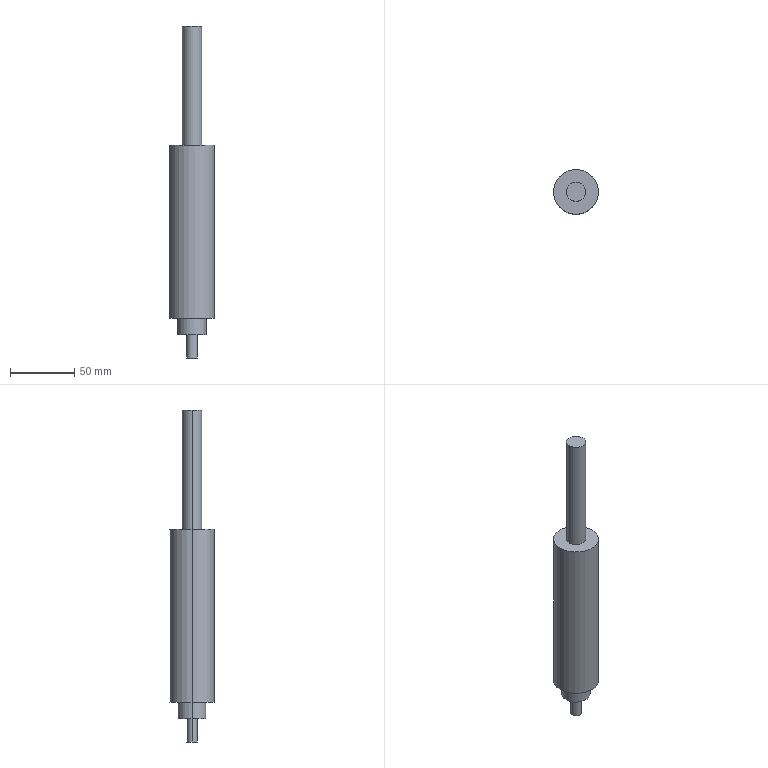Part | 1 solid | 13 faces | box 35 x 35 x 259 mm | volume 152166 mm3 | cylinder 8 | plane 5 | commonest cylinder face diameters 8 x2 15 x2 22 x2 35 x2
STEP:
#1=CARTESIAN_POINT('',(7.5,0.,259.));
#2=VERTEX_POINT('',#1);
#3=CARTESIAN_POINT('',(-7.5,0.,259.));
#4=VERTEX_POINT('',#3);
#5=CARTESIAN_POINT('',(0.,0.,259.));
#6=DIRECTION('',(0.,0.,1.));
#7=DIRECTION('',(1.,0.,0.));
#8=AXIS2_PLACEMENT_3D('',#5,#6,#7);
#9=CIRCLE('',#8,7.5);
#10=EDGE_CURVE('',#2,#4,#9,.T.);
#11=ORIENTED_EDGE('',*,*,#10,.F.);
#12=CARTESIAN_POINT('',(7.5,0.,166.));
#13=VERTEX_POINT('',#12);
#14=CARTESIAN_POINT('',(7.5,0.,259.));
#15=DIRECTION('',(0.,0.,-1.));
#16=VECTOR('',#15,1000.);
#17=LINE('',#14,#16);
#18=EDGE_CURVE('',#2,#13,#17,.T.);
#19=ORIENTED_EDGE('',*,*,#18,.T.);
#20=CARTESIAN_POINT('',(-7.5,0.,166.));
#21=VERTEX_POINT('',#20);
#22=CARTESIAN_POINT('',(0.,0.,166.));
#23=DIRECTION('',(0.,0.,1.));
#24=DIRECTION('',(1.,0.,0.));
#25=AXIS2_PLACEMENT_3D('',#22,#23,#24);
#26=CIRCLE('',#25,7.5);
#27=EDGE_CURVE('',#13,#21,#26,.T.);
#28=ORIENTED_EDGE('',*,*,#27,.T.);
#29=CARTESIAN_POINT('',(-7.5,0.,259.));
#30=DIRECTION('',(0.,0.,-1.));
#31=VECTOR('',#30,1000.);
#32=LINE('',#29,#31);
#33=EDGE_CURVE('',#4,#21,#32,.T.);
#34=ORIENTED_EDGE('',*,*,#33,.F.);
#35=EDGE_LOOP('',(#11,#19,#28,#34));
#36=FACE_OUTER_BOUND('',#35,.T.);
#37=CARTESIAN_POINT('',(0.,0.,259.));
#38=DIRECTION('',(0.,0.,-1.));
#39=DIRECTION('',(-1.,0.,0.));
#40=AXIS2_PLACEMENT_3D('',#37,#38,#39);
#41=CYLINDRICAL_SURFACE('',#40,7.5);
#42=ADVANCED_FACE('',(#36),#41,.T.);
#43=CARTESIAN_POINT('',(17.5,0.,166.));
#44=VERTEX_POINT('',#43);
#45=CARTESIAN_POINT('',(-17.5,0.,166.));
#46=VERTEX_POINT('',#45);
#47=CARTESIAN_POINT('',(0.,0.,166.));
#48=DIRECTION('',(0.,0.,1.));
#49=DIRECTION('',(1.,0.,0.));
#50=AXIS2_PLACEMENT_3D('',#47,#48,#49);
#51=CIRCLE('',#50,17.5);
#52=EDGE_CURVE('',#44,#46,#51,.T.);
#53=ORIENTED_EDGE('',*,*,#52,.F.);
#54=CARTESIAN_POINT('',(17.5,0.,31.));
#55=VERTEX_POINT('',#54);
#56=CARTESIAN_POINT('',(17.5,0.,166.));
#57=DIRECTION('',(0.,0.,-1.));
#58=VECTOR('',#57,1000.);
#59=LINE('',#56,#58);
#60=EDGE_CURVE('',#44,#55,#59,.T.);
#61=ORIENTED_EDGE('',*,*,#60,.T.);
#62=CARTESIAN_POINT('',(-17.5,0.,31.));
#63=VERTEX_POINT('',#62);
#64=CARTESIAN_POINT('',(0.,0.,31.));
#65=DIRECTION('',(0.,0.,1.));
#66=DIRECTION('',(1.,0.,0.));
#67=AXIS2_PLACEMENT_3D('',#64,#65,#66);
#68=CIRCLE('',#67,17.5);
#69=EDGE_CURVE('',#55,#63,#68,.T.);
#70=ORIENTED_EDGE('',*,*,#69,.T.);
#71=CARTESIAN_POINT('',(-17.5,0.,166.));
#72=DIRECTION('',(0.,0.,-1.));
#73=VECTOR('',#72,1000.);
#74=LINE('',#71,#73);
#75=EDGE_CURVE('',#46,#63,#74,.T.);
#76=ORIENTED_EDGE('',*,*,#75,.F.);
#77=EDGE_LOOP('',(#53,#61,#70,#76));
#78=FACE_OUTER_BOUND('',#77,.T.);
#79=CARTESIAN_POINT('',(0.,0.,166.));
#80=DIRECTION('',(0.,0.,-1.));
#81=DIRECTION('',(-1.,0.,0.));
#82=AXIS2_PLACEMENT_3D('',#79,#80,#81);
#83=CYLINDRICAL_SURFACE('',#82,17.5);
#84=ADVANCED_FACE('',(#78),#83,.T.);
#85=CARTESIAN_POINT('',(11.,0.,31.));
#86=VERTEX_POINT('',#85);
#87=CARTESIAN_POINT('',(-11.,0.,31.));
#88=VERTEX_POINT('',#87);
#89=CARTESIAN_POINT('',(0.,0.,31.));
#90=DIRECTION('',(0.,0.,1.));
#91=DIRECTION('',(1.,0.,0.));
#92=AXIS2_PLACEMENT_3D('',#89,#90,#91);
#93=CIRCLE('',#92,11.);
#94=EDGE_CURVE('',#86,#88,#93,.T.);
#95=ORIENTED_EDGE('',*,*,#94,.F.);
#96=CARTESIAN_POINT('',(11.,0.,18.));
#97=VERTEX_POINT('',#96);
#98=CARTESIAN_POINT('',(11.,0.,31.));
#99=DIRECTION('',(0.,0.,-1.));
#100=VECTOR('',#99,1000.);
#101=LINE('',#98,#100);
#102=EDGE_CURVE('',#86,#97,#101,.T.);
#103=ORIENTED_EDGE('',*,*,#102,.T.);
#104=CARTESIAN_POINT('',(-11.,0.,18.));
#105=VERTEX_POINT('',#104);
#106=CARTESIAN_POINT('',(0.,0.,18.));
#107=DIRECTION('',(0.,0.,1.));
#108=DIRECTION('',(1.,0.,0.));
#109=AXIS2_PLACEMENT_3D('',#106,#107,#108);
#110=CIRCLE('',#109,11.);
#111=EDGE_CURVE('',#97,#105,#110,.T.);
#112=ORIENTED_EDGE('',*,*,#111,.T.);
#113=CARTESIAN_POINT('',(-11.,0.,31.));
#114=DIRECTION('',(0.,0.,-1.));
#115=VECTOR('',#114,1000.);
#116=LINE('',#113,#115);
#117=EDGE_CURVE('',#88,#105,#116,.T.);
#118=ORIENTED_EDGE('',*,*,#117,.F.);
#119=EDGE_LOOP('',(#95,#103,#112,#118));
#120=FACE_OUTER_BOUND('',#119,.T.);
#121=CARTESIAN_POINT('',(0.,0.,31.));
#122=DIRECTION('',(0.,0.,-1.));
#123=DIRECTION('',(-1.,0.,0.));
#124=AXIS2_PLACEMENT_3D('',#121,#122,#123);
#125=CYLINDRICAL_SURFACE('',#124,11.);
#126=ADVANCED_FACE('',(#120),#125,.T.);
#127=CARTESIAN_POINT('',(4.,0.,18.));
#128=VERTEX_POINT('',#127);
#129=CARTESIAN_POINT('',(-4.,0.,18.));
#130=VERTEX_POINT('',#129);
#131=CARTESIAN_POINT('',(0.,0.,18.));
#132=DIRECTION('',(0.,0.,1.));
#133=DIRECTION('',(1.,0.,0.));
#134=AXIS2_PLACEMENT_3D('',#131,#132,#133);
#135=CIRCLE('',#134,4.);
#136=EDGE_CURVE('',#128,#130,#135,.T.);
#137=ORIENTED_EDGE('',*,*,#136,.F.);
#138=CARTESIAN_POINT('',(4.,0.,0.));
#139=VERTEX_POINT('',#138);
#140=CARTESIAN_POINT('',(4.,0.,18.));
#141=DIRECTION('',(0.,0.,-1.));
#142=VECTOR('',#141,1000.);
#143=LINE('',#140,#142);
#144=EDGE_CURVE('',#128,#139,#143,.T.);
#145=ORIENTED_EDGE('',*,*,#144,.T.);
#146=CARTESIAN_POINT('',(-4.,0.,0.));
#147=VERTEX_POINT('',#146);
#148=CARTESIAN_POINT('',(0.,0.,0.));
#149=DIRECTION('',(0.,0.,1.));
#150=DIRECTION('',(1.,0.,0.));
#151=AXIS2_PLACEMENT_3D('',#148,#149,#150);
#152=CIRCLE('',#151,4.);
#153=EDGE_CURVE('',#139,#147,#152,.T.);
#154=ORIENTED_EDGE('',*,*,#153,.T.);
#155=CARTESIAN_POINT('',(-4.,0.,18.));
#156=DIRECTION('',(0.,0.,-1.));
#157=VECTOR('',#156,1000.);
#158=LINE('',#155,#157);
#159=EDGE_CURVE('',#130,#147,#158,.T.);
#160=ORIENTED_EDGE('',*,*,#159,.F.);
#161=EDGE_LOOP('',(#137,#145,#154,#160));
#162=FACE_OUTER_BOUND('',#161,.T.);
#163=CARTESIAN_POINT('',(0.,0.,18.));
#164=DIRECTION('',(0.,0.,-1.));
#165=DIRECTION('',(-1.,0.,0.));
#166=AXIS2_PLACEMENT_3D('',#163,#164,#165);
#167=CYLINDRICAL_SURFACE('',#166,4.);
#168=ADVANCED_FACE('',(#162),#167,.T.);
#169=CARTESIAN_POINT('',(0.,0.,166.));
#170=DIRECTION('',(0.,0.,1.));
#171=DIRECTION('',(1.,0.,0.));
#172=AXIS2_PLACEMENT_3D('',#169,#170,#171);
#173=CIRCLE('',#172,17.5);
#174=EDGE_CURVE('',#46,#44,#173,.T.);
#175=ORIENTED_EDGE('',*,*,#174,.T.);
#176=ORIENTED_EDGE('',*,*,#52,.T.);
#177=EDGE_LOOP('',(#175,#176));
#178=FACE_OUTER_BOUND('',#177,.T.);
#179=CARTESIAN_POINT('',(0.,0.,166.));
#180=DIRECTION('',(0.,0.,1.));
#181=DIRECTION('',(1.,0.,0.));
#182=AXIS2_PLACEMENT_3D('',#179,#180,#181);
#183=CIRCLE('',#182,7.5);
#184=EDGE_CURVE('',#21,#13,#183,.T.);
#185=ORIENTED_EDGE('',*,*,#184,.F.);
#186=ORIENTED_EDGE('',*,*,#27,.F.);
#187=EDGE_LOOP('',(#185,#186));
#188=FACE_BOUND('',#187,.T.);
#189=CARTESIAN_POINT('',(0.,0.,166.));
#190=DIRECTION('',(0.,0.,1.));
#191=DIRECTION('',(1.,0.,0.));
#192=AXIS2_PLACEMENT_3D('',#189,#190,#191);
#193=PLANE('',#192);
#194=ADVANCED_FACE('',(#178,#188),#193,.T.);
#195=ORIENTED_EDGE('',*,*,#144,.F.);
#196=CARTESIAN_POINT('',(0.,0.,18.));
#197=DIRECTION('',(0.,0.,1.));
#198=DIRECTION('',(1.,0.,0.));
#199=AXIS2_PLACEMENT_3D('',#196,#197,#198);
#200=CIRCLE('',#199,4.);
#201=EDGE_CURVE('',#130,#128,#200,.T.);
#202=ORIENTED_EDGE('',*,*,#201,.F.);
#203=ORIENTED_EDGE('',*,*,#159,.T.);
#204=CARTESIAN_POINT('',(0.,0.,0.));
#205=DIRECTION('',(0.,0.,1.));
#206=DIRECTION('',(1.,0.,0.));
#207=AXIS2_PLACEMENT_3D('',#204,#205,#206);
#208=CIRCLE('',#207,4.);
#209=EDGE_CURVE('',#147,#139,#208,.T.);
#210=ORIENTED_EDGE('',*,*,#209,.T.);
#211=EDGE_LOOP('',(#195,#202,#203,#210));
#212=FACE_OUTER_BOUND('',#211,.T.);
#213=CARTESIAN_POINT('',(0.,0.,18.));
#214=DIRECTION('',(0.,0.,-1.));
#215=DIRECTION('',(-1.,0.,0.));
#216=AXIS2_PLACEMENT_3D('',#213,#214,#215);
#217=CYLINDRICAL_SURFACE('',#216,4.);
#218=ADVANCED_FACE('',(#212),#217,.T.);
#219=ORIENTED_EDGE('',*,*,#209,.F.);
#220=ORIENTED_EDGE('',*,*,#153,.F.);
#221=EDGE_LOOP('',(#219,#220));
#222=FACE_OUTER_BOUND('',#221,.T.);
#223=CARTESIAN_POINT('',(0.,0.,0.));
#224=DIRECTION('',(0.,0.,1.));
#225=DIRECTION('',(1.,0.,0.));
#226=AXIS2_PLACEMENT_3D('',#223,#224,#225);
#227=PLANE('',#226);
#228=ADVANCED_FACE('',(#222),#227,.F.);
#229=CARTESIAN_POINT('',(0.,0.,18.));
#230=DIRECTION('',(0.,0.,1.));
#231=DIRECTION('',(1.,0.,0.));
#232=AXIS2_PLACEMENT_3D('',#229,#230,#231);
#233=CIRCLE('',#232,11.);
#234=EDGE_CURVE('',#105,#97,#233,.T.);
#235=ORIENTED_EDGE('',*,*,#234,.F.);
#236=ORIENTED_EDGE('',*,*,#111,.F.);
#237=EDGE_LOOP('',(#235,#236));
#238=FACE_OUTER_BOUND('',#237,.T.);
#239=ORIENTED_EDGE('',*,*,#201,.T.);
#240=ORIENTED_EDGE('',*,*,#136,.T.);
#241=EDGE_LOOP('',(#239,#240));
#242=FACE_BOUND('',#241,.T.);
#243=CARTESIAN_POINT('',(0.,0.,18.));
#244=DIRECTION('',(0.,0.,1.));
#245=DIRECTION('',(1.,0.,0.));
#246=AXIS2_PLACEMENT_3D('',#243,#244,#245);
#247=PLANE('',#246);
#248=ADVANCED_FACE('',(#238,#242),#247,.F.);
#249=ORIENTED_EDGE('',*,*,#102,.F.);
#250=CARTESIAN_POINT('',(0.,0.,31.));
#251=DIRECTION('',(0.,0.,1.));
#252=DIRECTION('',(1.,0.,0.));
#253=AXIS2_PLACEMENT_3D('',#250,#251,#252);
#254=CIRCLE('',#253,11.);
#255=EDGE_CURVE('',#88,#86,#254,.T.);
#256=ORIENTED_EDGE('',*,*,#255,.F.);
#257=ORIENTED_EDGE('',*,*,#117,.T.);
#258=ORIENTED_EDGE('',*,*,#234,.T.);
#259=EDGE_LOOP('',(#249,#256,#257,#258));
#260=FACE_OUTER_BOUND('',#259,.T.);
#261=CARTESIAN_POINT('',(0.,0.,31.));
#262=DIRECTION('',(0.,0.,-1.));
#263=DIRECTION('',(-1.,0.,0.));
#264=AXIS2_PLACEMENT_3D('',#261,#262,#263);
#265=CYLINDRICAL_SURFACE('',#264,11.);
#266=ADVANCED_FACE('',(#260),#265,.T.);
#267=CARTESIAN_POINT('',(0.,0.,31.));
#268=DIRECTION('',(0.,0.,1.));
#269=DIRECTION('',(1.,0.,0.));
#270=AXIS2_PLACEMENT_3D('',#267,#268,#269);
#271=CIRCLE('',#270,17.5);
#272=EDGE_CURVE('',#63,#55,#271,.T.);
#273=ORIENTED_EDGE('',*,*,#272,.F.);
#274=ORIENTED_EDGE('',*,*,#69,.F.);
#275=EDGE_LOOP('',(#273,#274));
#276=FACE_OUTER_BOUND('',#275,.T.);
#277=ORIENTED_EDGE('',*,*,#255,.T.);
#278=ORIENTED_EDGE('',*,*,#94,.T.);
#279=EDGE_LOOP('',(#277,#278));
#280=FACE_BOUND('',#279,.T.);
#281=CARTESIAN_POINT('',(0.,0.,31.));
#282=DIRECTION('',(0.,0.,1.));
#283=DIRECTION('',(1.,0.,0.));
#284=AXIS2_PLACEMENT_3D('',#281,#282,#283);
#285=PLANE('',#284);
#286=ADVANCED_FACE('',(#276,#280),#285,.F.);
#287=ORIENTED_EDGE('',*,*,#60,.F.);
#288=ORIENTED_EDGE('',*,*,#174,.F.);
#289=ORIENTED_EDGE('',*,*,#75,.T.);
#290=ORIENTED_EDGE('',*,*,#272,.T.);
#291=EDGE_LOOP('',(#287,#288,#289,#290));
#292=FACE_OUTER_BOUND('',#291,.T.);
#293=CARTESIAN_POINT('',(0.,0.,166.));
#294=DIRECTION('',(0.,0.,-1.));
#295=DIRECTION('',(-1.,0.,0.));
#296=AXIS2_PLACEMENT_3D('',#293,#294,#295);
#297=CYLINDRICAL_SURFACE('',#296,17.5);
#298=ADVANCED_FACE('',(#292),#297,.T.);
#299=ORIENTED_EDGE('',*,*,#18,.F.);
#300=CARTESIAN_POINT('',(0.,0.,259.));
#301=DIRECTION('',(0.,0.,1.));
#302=DIRECTION('',(1.,0.,0.));
#303=AXIS2_PLACEMENT_3D('',#300,#301,#302);
#304=CIRCLE('',#303,7.5);
#305=EDGE_CURVE('',#4,#2,#304,.T.);
#306=ORIENTED_EDGE('',*,*,#305,.F.);
#307=ORIENTED_EDGE('',*,*,#33,.T.);
#308=ORIENTED_EDGE('',*,*,#184,.T.);
#309=EDGE_LOOP('',(#299,#306,#307,#308));
#310=FACE_OUTER_BOUND('',#309,.T.);
#311=CARTESIAN_POINT('',(0.,0.,259.));
#312=DIRECTION('',(0.,0.,-1.));
#313=DIRECTION('',(-1.,0.,0.));
#314=AXIS2_PLACEMENT_3D('',#311,#312,#313);
#315=CYLINDRICAL_SURFACE('',#314,7.5);
#316=ADVANCED_FACE('',(#310),#315,.T.);
#317=ORIENTED_EDGE('',*,*,#305,.T.);
#318=ORIENTED_EDGE('',*,*,#10,.T.);
#319=EDGE_LOOP('',(#317,#318));
#320=FACE_OUTER_BOUND('',#319,.T.);
#321=CARTESIAN_POINT('',(0.,0.,259.));
#322=DIRECTION('',(0.,0.,1.));
#323=DIRECTION('',(1.,0.,0.));
#324=AXIS2_PLACEMENT_3D('',#321,#322,#323);
#325=PLANE('',#324);
#326=ADVANCED_FACE('',(#320),#325,.T.);
#327=CLOSED_SHELL('',(#42,#84,#126,#168,#194,#218,#228,#248,#266,#286,#298,#316,#326));
#328=MANIFOLD_SOLID_BREP('',#327);
#329=CARTESIAN_POINT('',(0.,0.,0.));
#330=DIRECTION('',(0.,0.,1.));
#331=DIRECTION('',(1.,0.,0.));
#332=AXIS2_PLACEMENT_3D('',#329,#330,#331);
#333=(LENGTH_UNIT()NAMED_UNIT(*)SI_UNIT(.MILLI.,.METRE.));
#334=UNCERTAINTY_MEASURE_WITH_UNIT(LENGTH_MEASURE(0.00001),#333,'','');
#335=(NAMED_UNIT(*)PLANE_ANGLE_UNIT()SI_UNIT($,.RADIAN.));
#336=(NAMED_UNIT(*)SI_UNIT($,.STERADIAN.)SOLID_ANGLE_UNIT());
#337=(GEOMETRIC_REPRESENTATION_CONTEXT(3)GLOBAL_UNCERTAINTY_ASSIGNED_CONTEXT((#334))GLOBAL_UNIT_ASSIGNED_CONTEXT((#333,#335,#336))REPRESENTATION_CONTEXT('',''));
#338=ADVANCED_BREP_SHAPE_REPRESENTATION('',(#328,#332),#337);